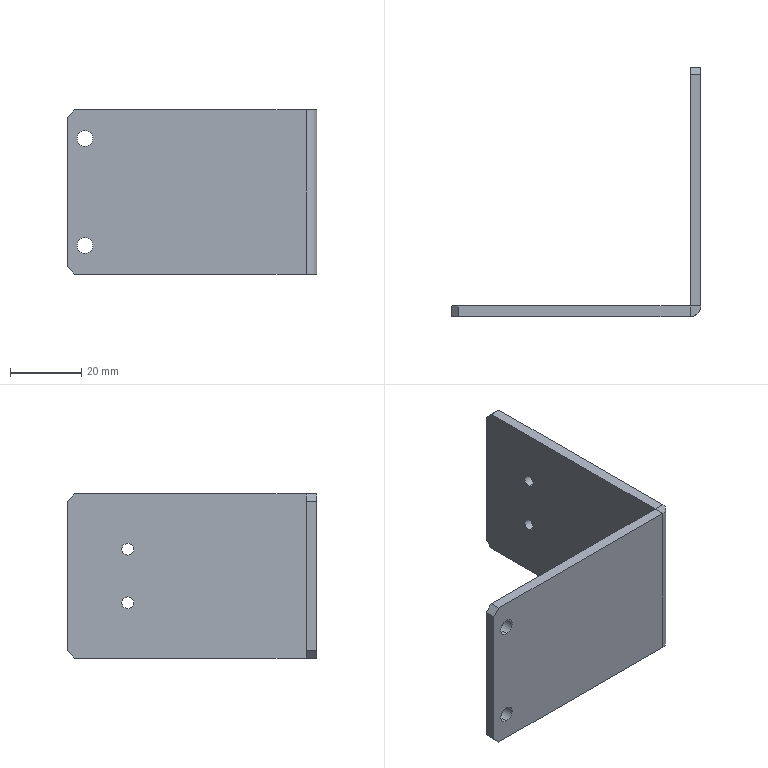Part | NX | features BREP 1 | 1 solid | 26 faces | box 70 x 70 x 46 mm | volume 18646 mm3 | plane 16 | cylinder 10 | commonest cylinder face diameters 3.3 x4 4.5 x4 0.02 x1 6.02 x1
STEP:
#1=CARTESIAN_POINT('',(0.,53.,5.85));
#2=VERTEX_POINT('',#1);
#3=CARTESIAN_POINT('',(0.,53.,9.15));
#4=VERTEX_POINT('',#3);
#5=CARTESIAN_POINT('',(0.,53.,7.5));
#6=DIRECTION('',(-1.,0.,0.));
#7=DIRECTION('',(0.,0.,1.));
#8=AXIS2_PLACEMENT_3D('',#5,#6,#7);
#9=CIRCLE('',#8,1.65);
#10=EDGE_CURVE('',#2,#4,#9,.T.);
#11=ORIENTED_EDGE('',*,*,#10,.F.);
#12=CARTESIAN_POINT('',(-3.,53.,5.85));
#13=VERTEX_POINT('',#12);
#14=CARTESIAN_POINT('',(-3.,53.,5.85));
#15=DIRECTION('',(-1.,0.,0.));
#16=VECTOR('',#15,1000.);
#17=LINE('',#14,#16);
#18=EDGE_CURVE('',#13,#2,#17,.F.);
#19=ORIENTED_EDGE('',*,*,#18,.F.);
#20=CARTESIAN_POINT('',(-3.,53.,9.15));
#21=VERTEX_POINT('',#20);
#22=CARTESIAN_POINT('',(-3.,53.,7.5));
#23=DIRECTION('',(-1.,0.,0.));
#24=DIRECTION('',(0.,0.,1.));
#25=AXIS2_PLACEMENT_3D('',#22,#23,#24);
#26=CIRCLE('',#25,1.65);
#27=EDGE_CURVE('',#13,#21,#26,.T.);
#28=ORIENTED_EDGE('',*,*,#27,.T.);
#29=CARTESIAN_POINT('',(-3.,53.,9.15));
#30=DIRECTION('',(-1.,0.,0.));
#31=VECTOR('',#30,1000.);
#32=LINE('',#29,#31);
#33=EDGE_CURVE('',#21,#4,#32,.F.);
#34=ORIENTED_EDGE('',*,*,#33,.T.);
#35=EDGE_LOOP('',(#11,#19,#28,#34));
#36=FACE_BOUND('',#35,.T.);
#37=CARTESIAN_POINT('',(-3.,53.,7.5));
#38=DIRECTION('',(-1.,0.,0.));
#39=DIRECTION('',(0.,0.,1.));
#40=AXIS2_PLACEMENT_3D('',#37,#38,#39);
#41=CYLINDRICAL_SURFACE('',#40,1.65);
#42=ADVANCED_FACE('',(#36),#41,.F.);
#43=CARTESIAN_POINT('',(0.,53.,-9.15));
#44=VERTEX_POINT('',#43);
#45=CARTESIAN_POINT('',(0.,53.,-5.85));
#46=VERTEX_POINT('',#45);
#47=CARTESIAN_POINT('',(0.,53.,-7.5));
#48=DIRECTION('',(-1.,0.,0.));
#49=DIRECTION('',(0.,0.,1.));
#50=AXIS2_PLACEMENT_3D('',#47,#48,#49);
#51=CIRCLE('',#50,1.65);
#52=EDGE_CURVE('',#44,#46,#51,.T.);
#53=ORIENTED_EDGE('',*,*,#52,.F.);
#54=CARTESIAN_POINT('',(-3.,53.,-9.15));
#55=VERTEX_POINT('',#54);
#56=CARTESIAN_POINT('',(-3.,53.,-9.15));
#57=DIRECTION('',(-1.,0.,0.));
#58=VECTOR('',#57,1000.);
#59=LINE('',#56,#58);
#60=EDGE_CURVE('',#55,#44,#59,.F.);
#61=ORIENTED_EDGE('',*,*,#60,.F.);
#62=CARTESIAN_POINT('',(-3.,53.,-5.85));
#63=VERTEX_POINT('',#62);
#64=CARTESIAN_POINT('',(-3.,53.,-7.5));
#65=DIRECTION('',(-1.,0.,0.));
#66=DIRECTION('',(0.,0.,1.));
#67=AXIS2_PLACEMENT_3D('',#64,#65,#66);
#68=CIRCLE('',#67,1.65);
#69=EDGE_CURVE('',#55,#63,#68,.T.);
#70=ORIENTED_EDGE('',*,*,#69,.T.);
#71=CARTESIAN_POINT('',(-3.,53.,-5.85));
#72=DIRECTION('',(-1.,0.,0.));
#73=VECTOR('',#72,1000.);
#74=LINE('',#71,#73);
#75=EDGE_CURVE('',#63,#46,#74,.F.);
#76=ORIENTED_EDGE('',*,*,#75,.T.);
#77=EDGE_LOOP('',(#53,#61,#70,#76));
#78=FACE_BOUND('',#77,.T.);
#79=CARTESIAN_POINT('',(-3.,53.,-7.5));
#80=DIRECTION('',(-1.,0.,0.));
#81=DIRECTION('',(0.,0.,1.));
#82=AXIS2_PLACEMENT_3D('',#79,#80,#81);
#83=CYLINDRICAL_SURFACE('',#82,1.65);
#84=ADVANCED_FACE('',(#78),#83,.F.);
#85=CARTESIAN_POINT('',(-65.,0.,-12.75));
#86=VERTEX_POINT('',#85);
#87=CARTESIAN_POINT('',(-65.,0.,-17.25));
#88=VERTEX_POINT('',#87);
#89=CARTESIAN_POINT('',(-65.,0.,-15.));
#90=DIRECTION('',(0.,-1.,0.));
#91=DIRECTION('',(1.,0.,0.));
#92=AXIS2_PLACEMENT_3D('',#89,#90,#91);
#93=CIRCLE('',#92,2.25);
#94=EDGE_CURVE('',#86,#88,#93,.T.);
#95=ORIENTED_EDGE('',*,*,#94,.T.);
#96=CARTESIAN_POINT('',(-65.,3.,-17.25));
#97=VERTEX_POINT('',#96);
#98=CARTESIAN_POINT('',(-65.,3.,-17.25));
#99=DIRECTION('',(0.,1.,0.));
#100=VECTOR('',#99,1000.);
#101=LINE('',#98,#100);
#102=EDGE_CURVE('',#97,#88,#101,.F.);
#103=ORIENTED_EDGE('',*,*,#102,.F.);
#104=CARTESIAN_POINT('',(-65.,3.,-12.75));
#105=VERTEX_POINT('',#104);
#106=CARTESIAN_POINT('',(-65.,3.,-15.));
#107=DIRECTION('',(0.,1.,0.));
#108=DIRECTION('',(0.,0.,1.));
#109=AXIS2_PLACEMENT_3D('',#106,#107,#108);
#110=CIRCLE('',#109,2.25);
#111=EDGE_CURVE('',#97,#105,#110,.T.);
#112=ORIENTED_EDGE('',*,*,#111,.T.);
#113=CARTESIAN_POINT('',(-65.,3.,-12.75));
#114=DIRECTION('',(0.,1.,0.));
#115=VECTOR('',#114,1000.);
#116=LINE('',#113,#115);
#117=EDGE_CURVE('',#105,#86,#116,.F.);
#118=ORIENTED_EDGE('',*,*,#117,.T.);
#119=EDGE_LOOP('',(#95,#103,#112,#118));
#120=FACE_BOUND('',#119,.T.);
#121=CARTESIAN_POINT('',(-65.,3.,-15.));
#122=DIRECTION('',(0.,1.,0.));
#123=DIRECTION('',(0.,0.,1.));
#124=AXIS2_PLACEMENT_3D('',#121,#122,#123);
#125=CYLINDRICAL_SURFACE('',#124,2.25);
#126=ADVANCED_FACE('',(#120),#125,.F.);
#127=CARTESIAN_POINT('',(-65.,0.,17.25));
#128=VERTEX_POINT('',#127);
#129=CARTESIAN_POINT('',(-65.,0.,12.75));
#130=VERTEX_POINT('',#129);
#131=CARTESIAN_POINT('',(-65.,0.,15.));
#132=DIRECTION('',(0.,-1.,0.));
#133=DIRECTION('',(1.,0.,0.));
#134=AXIS2_PLACEMENT_3D('',#131,#132,#133);
#135=CIRCLE('',#134,2.25);
#136=EDGE_CURVE('',#128,#130,#135,.T.);
#137=ORIENTED_EDGE('',*,*,#136,.T.);
#138=CARTESIAN_POINT('',(-65.,3.,12.75));
#139=VERTEX_POINT('',#138);
#140=CARTESIAN_POINT('',(-65.,3.,12.75));
#141=DIRECTION('',(0.,1.,0.));
#142=VECTOR('',#141,1000.);
#143=LINE('',#140,#142);
#144=EDGE_CURVE('',#139,#130,#143,.F.);
#145=ORIENTED_EDGE('',*,*,#144,.F.);
#146=CARTESIAN_POINT('',(-65.,3.,17.25));
#147=VERTEX_POINT('',#146);
#148=CARTESIAN_POINT('',(-65.,3.,15.));
#149=DIRECTION('',(0.,1.,0.));
#150=DIRECTION('',(0.,0.,1.));
#151=AXIS2_PLACEMENT_3D('',#148,#149,#150);
#152=CIRCLE('',#151,2.25);
#153=EDGE_CURVE('',#139,#147,#152,.T.);
#154=ORIENTED_EDGE('',*,*,#153,.T.);
#155=CARTESIAN_POINT('',(-65.,3.,17.25));
#156=DIRECTION('',(0.,1.,0.));
#157=VECTOR('',#156,1000.);
#158=LINE('',#155,#157);
#159=EDGE_CURVE('',#147,#128,#158,.F.);
#160=ORIENTED_EDGE('',*,*,#159,.T.);
#161=EDGE_LOOP('',(#137,#145,#154,#160));
#162=FACE_BOUND('',#161,.T.);
#163=CARTESIAN_POINT('',(-65.,3.,15.));
#164=DIRECTION('',(0.,1.,0.));
#165=DIRECTION('',(0.,0.,1.));
#166=AXIS2_PLACEMENT_3D('',#163,#164,#165);
#167=CYLINDRICAL_SURFACE('',#166,2.25);
#168=ADVANCED_FACE('',(#162),#167,.F.);
#169=CARTESIAN_POINT('',(-3.01,0.,23.));
#170=VERTEX_POINT('',#169);
#171=CARTESIAN_POINT('',(-3.01,3.,23.));
#172=VERTEX_POINT('',#171);
#173=CARTESIAN_POINT('',(-3.01,0.,23.));
#174=DIRECTION('',(0.,1.,0.));
#175=VECTOR('',#174,1000.);
#176=LINE('',#173,#175);
#177=EDGE_CURVE('',#170,#172,#176,.T.);
#178=ORIENTED_EDGE('',*,*,#177,.F.);
#179=CARTESIAN_POINT('',(0.,3.01,23.));
#180=VERTEX_POINT('',#179);
#181=CARTESIAN_POINT('',(-3.01,3.01,23.));
#182=DIRECTION('',(0.,0.,-1.));
#183=DIRECTION('',(1.,0.,0.));
#184=AXIS2_PLACEMENT_3D('',#181,#182,#183);
#185=CIRCLE('',#184,3.01);
#186=EDGE_CURVE('',#180,#170,#185,.T.);
#187=ORIENTED_EDGE('',*,*,#186,.F.);
#188=CARTESIAN_POINT('',(-3.,3.01,23.));
#189=VERTEX_POINT('',#188);
#190=CARTESIAN_POINT('',(-3.,3.01,23.));
#191=DIRECTION('',(1.,0.,0.));
#192=VECTOR('',#191,1000.);
#193=LINE('',#190,#192);
#194=EDGE_CURVE('',#189,#180,#193,.T.);
#195=ORIENTED_EDGE('',*,*,#194,.F.);
#196=CARTESIAN_POINT('',(-3.01,3.01,23.));
#197=DIRECTION('',(0.,0.,-1.));
#198=DIRECTION('',(1.,0.,0.));
#199=AXIS2_PLACEMENT_3D('',#196,#197,#198);
#200=CIRCLE('',#199,0.01);
#201=EDGE_CURVE('',#189,#172,#200,.T.);
#202=ORIENTED_EDGE('',*,*,#201,.T.);
#203=EDGE_LOOP('',(#178,#187,#195,#202));
#204=FACE_BOUND('',#203,.T.);
#205=CARTESIAN_POINT('',(-3.01,0.,23.));
#206=DIRECTION('',(0.,0.,1.));
#207=DIRECTION('',(1.,0.,0.));
#208=AXIS2_PLACEMENT_3D('',#205,#206,#207);
#209=PLANE('',#208);
#210=ADVANCED_FACE('',(#204),#209,.T.);
#211=CARTESIAN_POINT('',(-68.,3.,23.));
#212=VERTEX_POINT('',#211);
#213=CARTESIAN_POINT('',(0.,3.,23.));
#214=DIRECTION('',(-1.,0.,0.));
#215=VECTOR('',#214,1000.);
#216=LINE('',#213,#215);
#217=EDGE_CURVE('',#172,#212,#216,.T.);
#218=ORIENTED_EDGE('',*,*,#217,.T.);
#219=CARTESIAN_POINT('',(-68.,0.,23.));
#220=VERTEX_POINT('',#219);
#221=CARTESIAN_POINT('',(-68.,3.01,23.));
#222=DIRECTION('',(0.,-1.,0.));
#223=VECTOR('',#222,1000.);
#224=LINE('',#221,#223);
#225=EDGE_CURVE('',#212,#220,#224,.T.);
#226=ORIENTED_EDGE('',*,*,#225,.T.);
#227=CARTESIAN_POINT('',(0.,0.,23.));
#228=DIRECTION('',(-1.,0.,0.));
#229=VECTOR('',#228,1000.);
#230=LINE('',#227,#229);
#231=EDGE_CURVE('',#170,#220,#230,.T.);
#232=ORIENTED_EDGE('',*,*,#231,.F.);
#233=ORIENTED_EDGE('',*,*,#177,.T.);
#234=EDGE_LOOP('',(#218,#226,#232,#233));
#235=FACE_BOUND('',#234,.T.);
#236=CARTESIAN_POINT('',(-3.,3.01,23.));
#237=DIRECTION('',(0.,0.,1.));
#238=DIRECTION('',(1.,0.,0.));
#239=AXIS2_PLACEMENT_3D('',#236,#237,#238);
#240=PLANE('',#239);
#241=ADVANCED_FACE('',(#235),#240,.T.);
#242=CARTESIAN_POINT('',(0.,3.01,-23.));
#243=VERTEX_POINT('',#242);
#244=CARTESIAN_POINT('',(-3.,3.01,-23.));
#245=VERTEX_POINT('',#244);
#246=CARTESIAN_POINT('',(0.,3.01,-23.));
#247=DIRECTION('',(-1.,0.,0.));
#248=VECTOR('',#247,1000.);
#249=LINE('',#246,#248);
#250=EDGE_CURVE('',#243,#245,#249,.T.);
#251=ORIENTED_EDGE('',*,*,#250,.F.);
#252=CARTESIAN_POINT('',(-3.01,0.,-23.));
#253=VERTEX_POINT('',#252);
#254=CARTESIAN_POINT('',(-3.01,3.01,-23.));
#255=DIRECTION('',(0.,0.,-1.));
#256=DIRECTION('',(1.,0.,0.));
#257=AXIS2_PLACEMENT_3D('',#254,#255,#256);
#258=CIRCLE('',#257,3.01);
#259=EDGE_CURVE('',#243,#253,#258,.T.);
#260=ORIENTED_EDGE('',*,*,#259,.T.);
#261=CARTESIAN_POINT('',(-3.01,3.,-23.));
#262=VERTEX_POINT('',#261);
#263=CARTESIAN_POINT('',(-3.01,3.,-23.));
#264=DIRECTION('',(0.,-1.,0.));
#265=VECTOR('',#264,1000.);
#266=LINE('',#263,#265);
#267=EDGE_CURVE('',#262,#253,#266,.T.);
#268=ORIENTED_EDGE('',*,*,#267,.F.);
#269=CARTESIAN_POINT('',(-3.01,3.01,-23.));
#270=DIRECTION('',(0.,0.,-1.));
#271=DIRECTION('',(1.,0.,0.));
#272=AXIS2_PLACEMENT_3D('',#269,#270,#271);
#273=CIRCLE('',#272,0.01);
#274=EDGE_CURVE('',#245,#262,#273,.T.);
#275=ORIENTED_EDGE('',*,*,#274,.F.);
#276=EDGE_LOOP('',(#251,#260,#268,#275));
#277=FACE_BOUND('',#276,.T.);
#278=CARTESIAN_POINT('',(0.,3.01,-23.));
#279=DIRECTION('',(0.,0.,-1.));
#280=DIRECTION('',(0.,-1.,0.));
#281=AXIS2_PLACEMENT_3D('',#278,#279,#280);
#282=PLANE('',#281);
#283=ADVANCED_FACE('',(#277),#282,.T.);
#284=CARTESIAN_POINT('',(-3.,68.,-23.));
#285=VERTEX_POINT('',#284);
#286=CARTESIAN_POINT('',(-3.,70.,-23.));
#287=DIRECTION('',(0.,-1.,0.));
#288=VECTOR('',#287,1000.);
#289=LINE('',#286,#288);
#290=EDGE_CURVE('',#285,#245,#289,.T.);
#291=ORIENTED_EDGE('',*,*,#290,.F.);
#292=CARTESIAN_POINT('',(0.,68.,-23.));
#293=VERTEX_POINT('',#292);
#294=CARTESIAN_POINT('',(-3.01,68.,-23.));
#295=DIRECTION('',(1.,0.,0.));
#296=VECTOR('',#295,1000.);
#297=LINE('',#294,#296);
#298=EDGE_CURVE('',#285,#293,#297,.T.);
#299=ORIENTED_EDGE('',*,*,#298,.T.);
#300=CARTESIAN_POINT('',(0.,70.,-23.));
#301=DIRECTION('',(0.,-1.,0.));
#302=VECTOR('',#301,1000.);
#303=LINE('',#300,#302);
#304=EDGE_CURVE('',#293,#243,#303,.T.);
#305=ORIENTED_EDGE('',*,*,#304,.T.);
#306=ORIENTED_EDGE('',*,*,#250,.T.);
#307=EDGE_LOOP('',(#291,#299,#305,#306));
#308=FACE_BOUND('',#307,.T.);
#309=CARTESIAN_POINT('',(-3.01,3.,-23.));
#310=DIRECTION('',(0.,0.,-1.));
#311=DIRECTION('',(0.,-1.,0.));
#312=AXIS2_PLACEMENT_3D('',#309,#310,#311);
#313=PLANE('',#312);
#314=ADVANCED_FACE('',(#308),#313,.T.);
#315=CARTESIAN_POINT('',(-70.,3.,21.));
#316=VERTEX_POINT('',#315);
#317=CARTESIAN_POINT('',(-70.,3.,-21.));
#318=VERTEX_POINT('',#317);
#319=CARTESIAN_POINT('',(-70.,3.,23.));
#320=DIRECTION('',(0.,0.,-1.));
#321=VECTOR('',#320,1000.);
#322=LINE('',#319,#321);
#323=EDGE_CURVE('',#316,#318,#322,.T.);
#324=ORIENTED_EDGE('',*,*,#323,.F.);
#325=CARTESIAN_POINT('',(-70.,3.,21.));
#326=DIRECTION('',(0.7071,0.,0.7071));
#327=VECTOR('',#326,1000.);
#328=LINE('',#325,#327);
#329=EDGE_CURVE('',#316,#212,#328,.T.);
#330=ORIENTED_EDGE('',*,*,#329,.T.);
#331=ORIENTED_EDGE('',*,*,#217,.F.);
#332=CARTESIAN_POINT('',(-3.01,3.,23.));
#333=DIRECTION('',(0.,0.,-1.));
#334=VECTOR('',#333,1000.);
#335=LINE('',#332,#334);
#336=EDGE_CURVE('',#172,#262,#335,.T.);
#337=ORIENTED_EDGE('',*,*,#336,.T.);
#338=CARTESIAN_POINT('',(-68.,3.,-23.));
#339=VERTEX_POINT('',#338);
#340=CARTESIAN_POINT('',(0.,3.,-23.));
#341=DIRECTION('',(-1.,0.,0.));
#342=VECTOR('',#341,1000.);
#343=LINE('',#340,#342);
#344=EDGE_CURVE('',#262,#339,#343,.T.);
#345=ORIENTED_EDGE('',*,*,#344,.T.);
#346=CARTESIAN_POINT('',(-68.,3.,-23.));
#347=DIRECTION('',(-0.7071,0.,0.7071));
#348=VECTOR('',#347,1000.);
#349=LINE('',#346,#348);
#350=EDGE_CURVE('',#339,#318,#349,.T.);
#351=ORIENTED_EDGE('',*,*,#350,.T.);
#352=EDGE_LOOP('',(#324,#330,#331,#337,#345,#351));
#353=FACE_BOUND('',#352,.T.);
#354=CARTESIAN_POINT('',(-65.,3.,-15.));
#355=DIRECTION('',(0.,1.,0.));
#356=DIRECTION('',(0.,0.,1.));
#357=AXIS2_PLACEMENT_3D('',#354,#355,#356);
#358=CIRCLE('',#357,2.25);
#359=EDGE_CURVE('',#105,#97,#358,.T.);
#360=ORIENTED_EDGE('',*,*,#359,.F.);
#361=ORIENTED_EDGE('',*,*,#111,.F.);
#362=EDGE_LOOP('',(#360,#361));
#363=FACE_BOUND('',#362,.T.);
#364=CARTESIAN_POINT('',(-65.,3.,15.));
#365=DIRECTION('',(0.,1.,0.));
#366=DIRECTION('',(0.,0.,1.));
#367=AXIS2_PLACEMENT_3D('',#364,#365,#366);
#368=CIRCLE('',#367,2.25);
#369=EDGE_CURVE('',#147,#139,#368,.T.);
#370=ORIENTED_EDGE('',*,*,#369,.F.);
#371=ORIENTED_EDGE('',*,*,#153,.F.);
#372=EDGE_LOOP('',(#370,#371));
#373=FACE_BOUND('',#372,.T.);
#374=CARTESIAN_POINT('',(0.,3.,23.));
#375=DIRECTION('',(0.,-1.,0.));
#376=DIRECTION('',(0.,0.,-1.));
#377=AXIS2_PLACEMENT_3D('',#374,#375,#376);
#378=PLANE('',#377);
#379=ADVANCED_FACE('',(#353,#363,#373),#378,.F.);
#380=CARTESIAN_POINT('',(-70.,0.,21.));
#381=VERTEX_POINT('',#380);
#382=CARTESIAN_POINT('',(-70.,0.,-21.));
#383=VERTEX_POINT('',#382);
#384=CARTESIAN_POINT('',(-70.,0.,23.));
#385=DIRECTION('',(0.,0.,-1.));
#386=VECTOR('',#385,1000.);
#387=LINE('',#384,#386);
#388=EDGE_CURVE('',#381,#383,#387,.T.);
#389=ORIENTED_EDGE('',*,*,#388,.F.);
#390=CARTESIAN_POINT('',(-70.,0.,21.));
#391=DIRECTION('',(0.,1.,0.));
#392=VECTOR('',#391,1000.);
#393=LINE('',#390,#392);
#394=EDGE_CURVE('',#381,#316,#393,.T.);
#395=ORIENTED_EDGE('',*,*,#394,.T.);
#396=ORIENTED_EDGE('',*,*,#323,.T.);
#397=CARTESIAN_POINT('',(-70.,0.,-21.));
#398=DIRECTION('',(0.,-1.,0.));
#399=VECTOR('',#398,1000.);
#400=LINE('',#397,#399);
#401=EDGE_CURVE('',#318,#383,#400,.T.);
#402=ORIENTED_EDGE('',*,*,#401,.T.);
#403=EDGE_LOOP('',(#389,#395,#396,#402));
#404=FACE_BOUND('',#403,.T.);
#405=CARTESIAN_POINT('',(-70.,0.,23.));
#406=DIRECTION('',(-1.,0.,0.));
#407=DIRECTION('',(0.,0.,1.));
#408=AXIS2_PLACEMENT_3D('',#405,#406,#407);
#409=PLANE('',#408);
#410=ADVANCED_FACE('',(#404),#409,.T.);
#411=ORIENTED_EDGE('',*,*,#231,.T.);
#412=CARTESIAN_POINT('',(-34.,0.,57.));
#413=DIRECTION('',(-0.7071,0.,-0.7071));
#414=VECTOR('',#413,1000.);
#415=LINE('',#412,#414);
#416=EDGE_CURVE('',#220,#381,#415,.T.);
#417=ORIENTED_EDGE('',*,*,#416,.T.);
#418=ORIENTED_EDGE('',*,*,#388,.T.);
#419=CARTESIAN_POINT('',(-68.,0.,-23.));
#420=VERTEX_POINT('',#419);
#421=CARTESIAN_POINT('',(-57.,0.,-34.));
#422=DIRECTION('',(0.7071,0.,-0.7071));
#423=VECTOR('',#422,1000.);
#424=LINE('',#421,#423);
#425=EDGE_CURVE('',#383,#420,#424,.T.);
#426=ORIENTED_EDGE('',*,*,#425,.T.);
#427=CARTESIAN_POINT('',(0.,0.,-23.));
#428=DIRECTION('',(-1.,0.,0.));
#429=VECTOR('',#428,1000.);
#430=LINE('',#427,#429);
#431=EDGE_CURVE('',#253,#420,#430,.T.);
#432=ORIENTED_EDGE('',*,*,#431,.F.);
#433=CARTESIAN_POINT('',(-3.01,0.,23.));
#434=DIRECTION('',(0.,0.,-1.));
#435=VECTOR('',#434,1000.);
#436=LINE('',#433,#435);
#437=EDGE_CURVE('',#170,#253,#436,.T.);
#438=ORIENTED_EDGE('',*,*,#437,.F.);
#439=EDGE_LOOP('',(#411,#417,#418,#426,#432,#438));
#440=FACE_BOUND('',#439,.T.);
#441=ORIENTED_EDGE('',*,*,#94,.F.);
#442=CARTESIAN_POINT('',(-65.,0.,-15.));
#443=DIRECTION('',(0.,-1.,0.));
#444=DIRECTION('',(1.,0.,0.));
#445=AXIS2_PLACEMENT_3D('',#442,#443,#444);
#446=CIRCLE('',#445,2.25);
#447=EDGE_CURVE('',#88,#86,#446,.T.);
#448=ORIENTED_EDGE('',*,*,#447,.F.);
#449=EDGE_LOOP('',(#441,#448));
#450=FACE_BOUND('',#449,.T.);
#451=ORIENTED_EDGE('',*,*,#136,.F.);
#452=CARTESIAN_POINT('',(-65.,0.,15.));
#453=DIRECTION('',(0.,-1.,0.));
#454=DIRECTION('',(1.,0.,0.));
#455=AXIS2_PLACEMENT_3D('',#452,#453,#454);
#456=CIRCLE('',#455,2.25);
#457=EDGE_CURVE('',#130,#128,#456,.T.);
#458=ORIENTED_EDGE('',*,*,#457,.F.);
#459=EDGE_LOOP('',(#451,#458));
#460=FACE_BOUND('',#459,.T.);
#461=CARTESIAN_POINT('',(0.,0.,23.));
#462=DIRECTION('',(0.,-1.,0.));
#463=DIRECTION('',(0.,0.,-1.));
#464=AXIS2_PLACEMENT_3D('',#461,#462,#463);
#465=PLANE('',#464);
#466=ADVANCED_FACE('',(#440,#450,#460),#465,.T.);
#467=ORIENTED_EDGE('',*,*,#259,.F.);
#468=CARTESIAN_POINT('',(0.,3.01,23.));
#469=DIRECTION('',(0.,0.,-1.));
#470=VECTOR('',#469,1000.);
#471=LINE('',#468,#470);
#472=EDGE_CURVE('',#180,#243,#471,.T.);
#473=ORIENTED_EDGE('',*,*,#472,.F.);
#474=ORIENTED_EDGE('',*,*,#186,.T.);
#475=ORIENTED_EDGE('',*,*,#437,.T.);
#476=EDGE_LOOP('',(#467,#473,#474,#475));
#477=FACE_BOUND('',#476,.T.);
#478=CARTESIAN_POINT('',(-3.01,3.01,23.));
#479=DIRECTION('',(0.,0.,-1.));
#480=DIRECTION('',(-1.,0.,0.));
#481=AXIS2_PLACEMENT_3D('',#478,#479,#480);
#482=CYLINDRICAL_SURFACE('',#481,3.01);
#483=ADVANCED_FACE('',(#477),#482,.T.);
#484=ORIENTED_EDGE('',*,*,#304,.F.);
#485=CARTESIAN_POINT('',(0.,70.,-21.));
#486=VERTEX_POINT('',#485);
#487=CARTESIAN_POINT('',(0.,92.,1.));
#488=DIRECTION('',(0.,0.7071,0.7071));
#489=VECTOR('',#488,1000.);
#490=LINE('',#487,#489);
#491=EDGE_CURVE('',#293,#486,#490,.T.);
#492=ORIENTED_EDGE('',*,*,#491,.T.);
#493=CARTESIAN_POINT('',(0.,70.,21.));
#494=VERTEX_POINT('',#493);
#495=CARTESIAN_POINT('',(0.,70.,23.));
#496=DIRECTION('',(0.,0.,-1.));
#497=VECTOR('',#496,1000.);
#498=LINE('',#495,#497);
#499=EDGE_CURVE('',#494,#486,#498,.T.);
#500=ORIENTED_EDGE('',*,*,#499,.F.);
#501=CARTESIAN_POINT('',(0.,68.,23.));
#502=VERTEX_POINT('',#501);
#503=CARTESIAN_POINT('',(0.,69.,22.));
#504=DIRECTION('',(0.,-0.7071,0.7071));
#505=VECTOR('',#504,1000.);
#506=LINE('',#503,#505);
#507=EDGE_CURVE('',#494,#502,#506,.T.);
#508=ORIENTED_EDGE('',*,*,#507,.T.);
#509=CARTESIAN_POINT('',(0.,70.,23.));
#510=DIRECTION('',(0.,-1.,0.));
#511=VECTOR('',#510,1000.);
#512=LINE('',#509,#511);
#513=EDGE_CURVE('',#502,#180,#512,.T.);
#514=ORIENTED_EDGE('',*,*,#513,.T.);
#515=ORIENTED_EDGE('',*,*,#472,.T.);
#516=EDGE_LOOP('',(#484,#492,#500,#508,#514,#515));
#517=FACE_BOUND('',#516,.T.);
#518=CARTESIAN_POINT('',(0.,53.,7.5));
#519=DIRECTION('',(-1.,0.,0.));
#520=DIRECTION('',(0.,0.,1.));
#521=AXIS2_PLACEMENT_3D('',#518,#519,#520);
#522=CIRCLE('',#521,1.65);
#523=EDGE_CURVE('',#4,#2,#522,.T.);
#524=ORIENTED_EDGE('',*,*,#523,.T.);
#525=ORIENTED_EDGE('',*,*,#10,.T.);
#526=EDGE_LOOP('',(#524,#525));
#527=FACE_BOUND('',#526,.T.);
#528=CARTESIAN_POINT('',(0.,53.,-7.5));
#529=DIRECTION('',(-1.,0.,0.));
#530=DIRECTION('',(0.,0.,1.));
#531=AXIS2_PLACEMENT_3D('',#528,#529,#530);
#532=CIRCLE('',#531,1.65);
#533=EDGE_CURVE('',#46,#44,#532,.T.);
#534=ORIENTED_EDGE('',*,*,#533,.T.);
#535=ORIENTED_EDGE('',*,*,#52,.T.);
#536=EDGE_LOOP('',(#534,#535));
#537=FACE_BOUND('',#536,.T.);
#538=CARTESIAN_POINT('',(0.,70.,23.));
#539=DIRECTION('',(1.,0.,0.));
#540=DIRECTION('',(0.,1.,0.));
#541=AXIS2_PLACEMENT_3D('',#538,#539,#540);
#542=PLANE('',#541);
#543=ADVANCED_FACE('',(#517,#527,#537),#542,.T.);
#544=ORIENTED_EDGE('',*,*,#499,.T.);
#545=CARTESIAN_POINT('',(-3.,70.,-21.));
#546=VERTEX_POINT('',#545);
#547=CARTESIAN_POINT('',(-3.,70.,-21.));
#548=DIRECTION('',(-1.,0.,0.));
#549=VECTOR('',#548,1000.);
#550=LINE('',#547,#549);
#551=EDGE_CURVE('',#486,#546,#550,.T.);
#552=ORIENTED_EDGE('',*,*,#551,.T.);
#553=CARTESIAN_POINT('',(-3.,70.,21.));
#554=VERTEX_POINT('',#553);
#555=CARTESIAN_POINT('',(-3.,70.,23.));
#556=DIRECTION('',(0.,0.,-1.));
#557=VECTOR('',#556,1000.);
#558=LINE('',#555,#557);
#559=EDGE_CURVE('',#554,#546,#558,.T.);
#560=ORIENTED_EDGE('',*,*,#559,.F.);
#561=CARTESIAN_POINT('',(-3.,70.,21.));
#562=DIRECTION('',(1.,0.,0.));
#563=VECTOR('',#562,1000.);
#564=LINE('',#561,#563);
#565=EDGE_CURVE('',#554,#494,#564,.T.);
#566=ORIENTED_EDGE('',*,*,#565,.T.);
#567=EDGE_LOOP('',(#544,#552,#560,#566));
#568=FACE_BOUND('',#567,.T.);
#569=CARTESIAN_POINT('',(-3.,70.,23.));
#570=DIRECTION('',(0.,1.,0.));
#571=DIRECTION('',(1.,0.,0.));
#572=AXIS2_PLACEMENT_3D('',#569,#570,#571);
#573=PLANE('',#572);
#574=ADVANCED_FACE('',(#568),#573,.T.);
#575=ORIENTED_EDGE('',*,*,#559,.T.);
#576=CARTESIAN_POINT('',(-3.,68.,-23.));
#577=DIRECTION('',(0.,-0.7071,-0.7071));
#578=VECTOR('',#577,1000.);
#579=LINE('',#576,#578);
#580=EDGE_CURVE('',#546,#285,#579,.T.);
#581=ORIENTED_EDGE('',*,*,#580,.T.);
#582=ORIENTED_EDGE('',*,*,#290,.T.);
#583=CARTESIAN_POINT('',(-3.,3.01,23.));
#584=DIRECTION('',(0.,0.,-1.));
#585=VECTOR('',#584,1000.);
#586=LINE('',#583,#585);
#587=EDGE_CURVE('',#189,#245,#586,.T.);
#588=ORIENTED_EDGE('',*,*,#587,.F.);
#589=CARTESIAN_POINT('',(-3.,68.,23.));
#590=VERTEX_POINT('',#589);
#591=CARTESIAN_POINT('',(-3.,70.,23.));
#592=DIRECTION('',(0.,-1.,0.));
#593=VECTOR('',#592,1000.);
#594=LINE('',#591,#593);
#595=EDGE_CURVE('',#590,#189,#594,.T.);
#596=ORIENTED_EDGE('',*,*,#595,.F.);
#597=CARTESIAN_POINT('',(-3.,70.,21.));
#598=DIRECTION('',(0.,0.7071,-0.7071));
#599=VECTOR('',#598,1000.);
#600=LINE('',#597,#599);
#601=EDGE_CURVE('',#590,#554,#600,.T.);
#602=ORIENTED_EDGE('',*,*,#601,.T.);
#603=EDGE_LOOP('',(#575,#581,#582,#588,#596,#602));
#604=FACE_BOUND('',#603,.T.);
#605=CARTESIAN_POINT('',(-3.,53.,7.5));
#606=DIRECTION('',(-1.,0.,0.));
#607=DIRECTION('',(0.,0.,1.));
#608=AXIS2_PLACEMENT_3D('',#605,#606,#607);
#609=CIRCLE('',#608,1.65);
#610=EDGE_CURVE('',#21,#13,#609,.T.);
#611=ORIENTED_EDGE('',*,*,#610,.F.);
#612=ORIENTED_EDGE('',*,*,#27,.F.);
#613=EDGE_LOOP('',(#611,#612));
#614=FACE_BOUND('',#613,.T.);
#615=CARTESIAN_POINT('',(-3.,53.,-7.5));
#616=DIRECTION('',(-1.,0.,0.));
#617=DIRECTION('',(0.,0.,1.));
#618=AXIS2_PLACEMENT_3D('',#615,#616,#617);
#619=CIRCLE('',#618,1.65);
#620=EDGE_CURVE('',#63,#55,#619,.T.);
#621=ORIENTED_EDGE('',*,*,#620,.F.);
#622=ORIENTED_EDGE('',*,*,#69,.F.);
#623=EDGE_LOOP('',(#621,#622));
#624=FACE_BOUND('',#623,.T.);
#625=CARTESIAN_POINT('',(-3.,70.,23.));
#626=DIRECTION('',(1.,0.,0.));
#627=DIRECTION('',(0.,1.,0.));
#628=AXIS2_PLACEMENT_3D('',#625,#626,#627);
#629=PLANE('',#628);
#630=ADVANCED_FACE('',(#604,#614,#624),#629,.F.);
#631=ORIENTED_EDGE('',*,*,#274,.T.);
#632=ORIENTED_EDGE('',*,*,#336,.F.);
#633=ORIENTED_EDGE('',*,*,#201,.F.);
#634=ORIENTED_EDGE('',*,*,#587,.T.);
#635=EDGE_LOOP('',(#631,#632,#633,#634));
#636=FACE_BOUND('',#635,.T.);
#637=CARTESIAN_POINT('',(-3.01,3.01,23.));
#638=DIRECTION('',(0.,0.,-1.));
#639=DIRECTION('',(-1.,0.,0.));
#640=AXIS2_PLACEMENT_3D('',#637,#638,#639);
#641=CYLINDRICAL_SURFACE('',#640,0.01);
#642=ADVANCED_FACE('',(#636),#641,.F.);
#643=ORIENTED_EDGE('',*,*,#513,.F.);
#644=CARTESIAN_POINT('',(-3.01,68.,23.));
#645=DIRECTION('',(-1.,0.,0.));
#646=VECTOR('',#645,1000.);
#647=LINE('',#644,#646);
#648=EDGE_CURVE('',#502,#590,#647,.T.);
#649=ORIENTED_EDGE('',*,*,#648,.T.);
#650=ORIENTED_EDGE('',*,*,#595,.T.);
#651=ORIENTED_EDGE('',*,*,#194,.T.);
#652=EDGE_LOOP('',(#643,#649,#650,#651));
#653=FACE_BOUND('',#652,.T.);
#654=CARTESIAN_POINT('',(-3.01,3.01,23.));
#655=DIRECTION('',(0.,0.,1.));
#656=DIRECTION('',(1.,0.,0.));
#657=AXIS2_PLACEMENT_3D('',#654,#655,#656);
#658=PLANE('',#657);
#659=ADVANCED_FACE('',(#653),#658,.T.);
#660=ORIENTED_EDGE('',*,*,#431,.T.);
#661=CARTESIAN_POINT('',(-68.,3.,-23.));
#662=DIRECTION('',(0.,1.,0.));
#663=VECTOR('',#662,1000.);
#664=LINE('',#661,#663);
#665=EDGE_CURVE('',#420,#339,#664,.T.);
#666=ORIENTED_EDGE('',*,*,#665,.T.);
#667=ORIENTED_EDGE('',*,*,#344,.F.);
#668=ORIENTED_EDGE('',*,*,#267,.T.);
#669=EDGE_LOOP('',(#660,#666,#667,#668));
#670=FACE_BOUND('',#669,.T.);
#671=CARTESIAN_POINT('',(-3.01,3.01,-23.));
#672=DIRECTION('',(0.,0.,1.));
#673=DIRECTION('',(1.,0.,0.));
#674=AXIS2_PLACEMENT_3D('',#671,#672,#673);
#675=PLANE('',#674);
#676=ADVANCED_FACE('',(#670),#675,.F.);
#677=ORIENTED_EDGE('',*,*,#144,.T.);
#678=ORIENTED_EDGE('',*,*,#457,.T.);
#679=ORIENTED_EDGE('',*,*,#159,.F.);
#680=ORIENTED_EDGE('',*,*,#369,.T.);
#681=EDGE_LOOP('',(#677,#678,#679,#680));
#682=FACE_BOUND('',#681,.T.);
#683=CARTESIAN_POINT('',(-65.,3.,15.));
#684=DIRECTION('',(0.,1.,0.));
#685=DIRECTION('',(0.,0.,1.));
#686=AXIS2_PLACEMENT_3D('',#683,#684,#685);
#687=CYLINDRICAL_SURFACE('',#686,2.25);
#688=ADVANCED_FACE('',(#682),#687,.F.);
#689=ORIENTED_EDGE('',*,*,#102,.T.);
#690=ORIENTED_EDGE('',*,*,#447,.T.);
#691=ORIENTED_EDGE('',*,*,#117,.F.);
#692=ORIENTED_EDGE('',*,*,#359,.T.);
#693=EDGE_LOOP('',(#689,#690,#691,#692));
#694=FACE_BOUND('',#693,.T.);
#695=CARTESIAN_POINT('',(-65.,3.,-15.));
#696=DIRECTION('',(0.,1.,0.));
#697=DIRECTION('',(0.,0.,1.));
#698=AXIS2_PLACEMENT_3D('',#695,#696,#697);
#699=CYLINDRICAL_SURFACE('',#698,2.25);
#700=ADVANCED_FACE('',(#694),#699,.F.);
#701=ORIENTED_EDGE('',*,*,#580,.F.);
#702=ORIENTED_EDGE('',*,*,#551,.F.);
#703=ORIENTED_EDGE('',*,*,#491,.F.);
#704=ORIENTED_EDGE('',*,*,#298,.F.);
#705=EDGE_LOOP('',(#701,#702,#703,#704));
#706=FACE_BOUND('',#705,.T.);
#707=CARTESIAN_POINT('',(-3.01,68.,-23.));
#708=DIRECTION('',(0.,-0.7071,0.7071));
#709=DIRECTION('',(-1.,0.,0.));
#710=AXIS2_PLACEMENT_3D('',#707,#708,#709);
#711=PLANE('',#710);
#712=ADVANCED_FACE('',(#706),#711,.F.);
#713=ORIENTED_EDGE('',*,*,#601,.F.);
#714=ORIENTED_EDGE('',*,*,#648,.F.);
#715=ORIENTED_EDGE('',*,*,#507,.F.);
#716=ORIENTED_EDGE('',*,*,#565,.F.);
#717=EDGE_LOOP('',(#713,#714,#715,#716));
#718=FACE_BOUND('',#717,.T.);
#719=CARTESIAN_POINT('',(-3.,70.,21.));
#720=DIRECTION('',(0.,-0.7071,-0.7071));
#721=DIRECTION('',(0.,-0.7071,0.7071));
#722=AXIS2_PLACEMENT_3D('',#719,#720,#721);
#723=PLANE('',#722);
#724=ADVANCED_FACE('',(#718),#723,.F.);
#725=ORIENTED_EDGE('',*,*,#416,.F.);
#726=ORIENTED_EDGE('',*,*,#225,.F.);
#727=ORIENTED_EDGE('',*,*,#329,.F.);
#728=ORIENTED_EDGE('',*,*,#394,.F.);
#729=EDGE_LOOP('',(#725,#726,#727,#728));
#730=FACE_BOUND('',#729,.T.);
#731=CARTESIAN_POINT('',(-70.,0.,21.));
#732=DIRECTION('',(0.7071,0.,-0.7071));
#733=DIRECTION('',(0.,-1.,0.));
#734=AXIS2_PLACEMENT_3D('',#731,#732,#733);
#735=PLANE('',#734);
#736=ADVANCED_FACE('',(#730),#735,.F.);
#737=ORIENTED_EDGE('',*,*,#425,.F.);
#738=ORIENTED_EDGE('',*,*,#401,.F.);
#739=ORIENTED_EDGE('',*,*,#350,.F.);
#740=ORIENTED_EDGE('',*,*,#665,.F.);
#741=EDGE_LOOP('',(#737,#738,#739,#740));
#742=FACE_BOUND('',#741,.T.);
#743=CARTESIAN_POINT('',(-68.,3.01,-23.));
#744=DIRECTION('',(-0.7071,0.,-0.7071));
#745=DIRECTION('',(-0.7071,0.,0.7071));
#746=AXIS2_PLACEMENT_3D('',#743,#744,#745);
#747=PLANE('',#746);
#748=ADVANCED_FACE('',(#742),#747,.T.);
#749=ORIENTED_EDGE('',*,*,#60,.T.);
#750=ORIENTED_EDGE('',*,*,#533,.F.);
#751=ORIENTED_EDGE('',*,*,#75,.F.);
#752=ORIENTED_EDGE('',*,*,#620,.T.);
#753=EDGE_LOOP('',(#749,#750,#751,#752));
#754=FACE_BOUND('',#753,.T.);
#755=CARTESIAN_POINT('',(-3.,53.,-7.5));
#756=DIRECTION('',(-1.,0.,0.));
#757=DIRECTION('',(0.,0.,1.));
#758=AXIS2_PLACEMENT_3D('',#755,#756,#757);
#759=CYLINDRICAL_SURFACE('',#758,1.65);
#760=ADVANCED_FACE('',(#754),#759,.F.);
#761=ORIENTED_EDGE('',*,*,#18,.T.);
#762=ORIENTED_EDGE('',*,*,#523,.F.);
#763=ORIENTED_EDGE('',*,*,#33,.F.);
#764=ORIENTED_EDGE('',*,*,#610,.T.);
#765=EDGE_LOOP('',(#761,#762,#763,#764));
#766=FACE_BOUND('',#765,.T.);
#767=CARTESIAN_POINT('',(-3.,53.,7.5));
#768=DIRECTION('',(-1.,0.,0.));
#769=DIRECTION('',(0.,0.,1.));
#770=AXIS2_PLACEMENT_3D('',#767,#768,#769);
#771=CYLINDRICAL_SURFACE('',#770,1.65);
#772=ADVANCED_FACE('',(#766),#771,.F.);
#773=CLOSED_SHELL('',(#42,#84,#126,#168,#210,#241,#283,#314,#379,#410,#466,#483,#543,#574,#630,#642,#659,#676,#688,#700,#712,#724,#736,#748,#760,#772));
#774=MANIFOLD_SOLID_BREP('',#773);
#775=(LENGTH_UNIT()NAMED_UNIT(*)SI_UNIT(.MILLI.,.METRE.));
#776=UNCERTAINTY_MEASURE_WITH_UNIT(LENGTH_MEASURE(0.00001),#775,'','');
#777=(NAMED_UNIT(*)PLANE_ANGLE_UNIT()SI_UNIT($,.RADIAN.));
#778=(NAMED_UNIT(*)SI_UNIT($,.STERADIAN.)SOLID_ANGLE_UNIT());
#779=(GEOMETRIC_REPRESENTATION_CONTEXT(3)GLOBAL_UNCERTAINTY_ASSIGNED_CONTEXT((#776))GLOBAL_UNIT_ASSIGNED_CONTEXT((#775,#777,#778))REPRESENTATION_CONTEXT('',''));
#780=ADVANCED_BREP_SHAPE_REPRESENTATION('',(#774),#779);